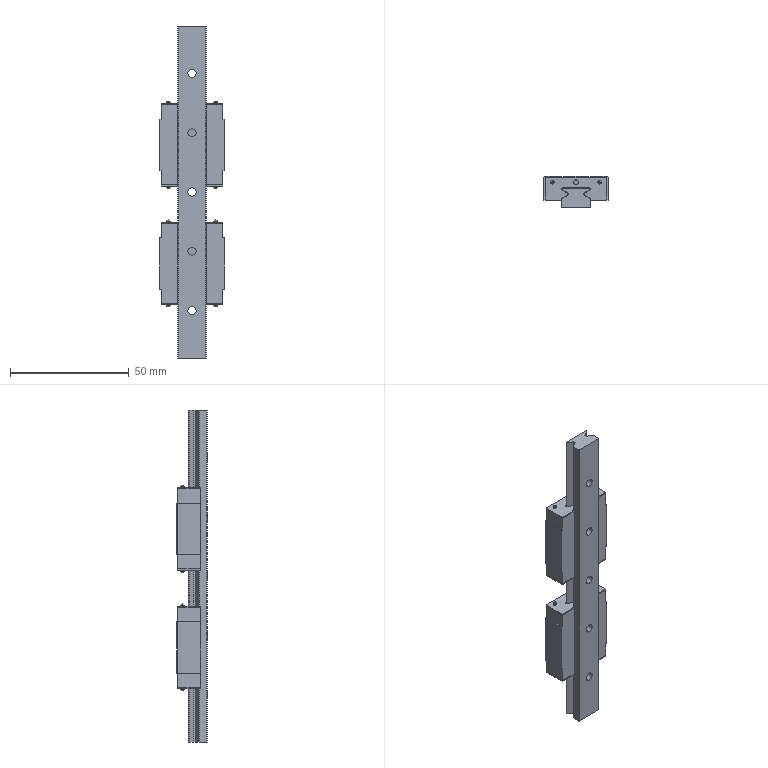Part | SolidWorks | features LocalLPattern 1, ReferencePattern 1 | 7 solids | 437 faces | box 27 x 13 x 140 mm | volume 25516 mm3 | plane 361 | cylinder 60 | sphere 16 | commonest cylinder face diameters 1.5 x16 3 x16 3.5 x10 6 x10 2 x8